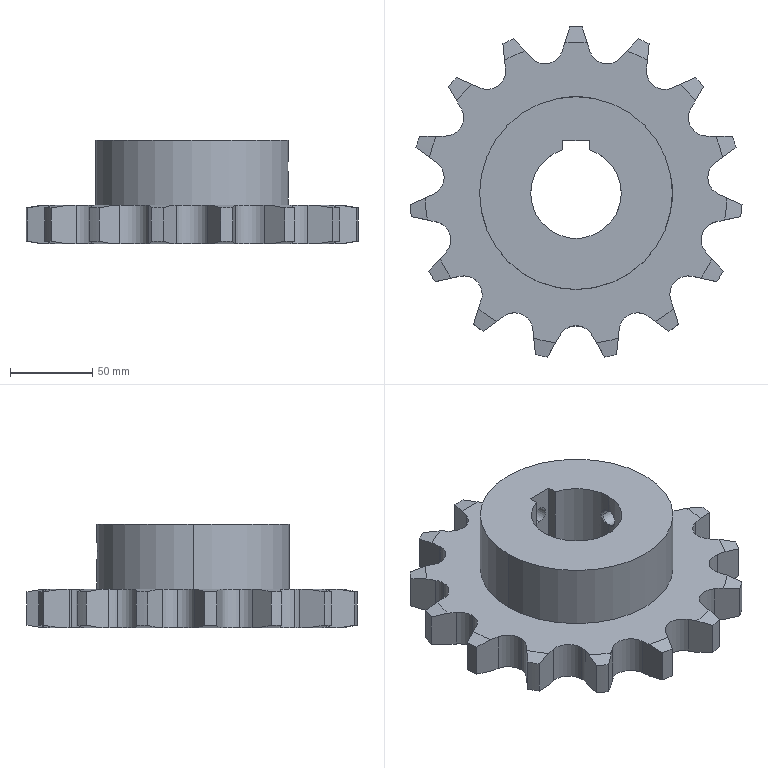Part | SolidWorks | features BaseBody 1 | 1 solid | 116 faces | box 201.53 x 200.494 x 63 mm | volume 849751 mm3 | cylinder 44 | cone 36 | plane 36 | commonest cylinder face diameters 22.23 x20 202 x15 10.106 x4 55 x3 117 x2